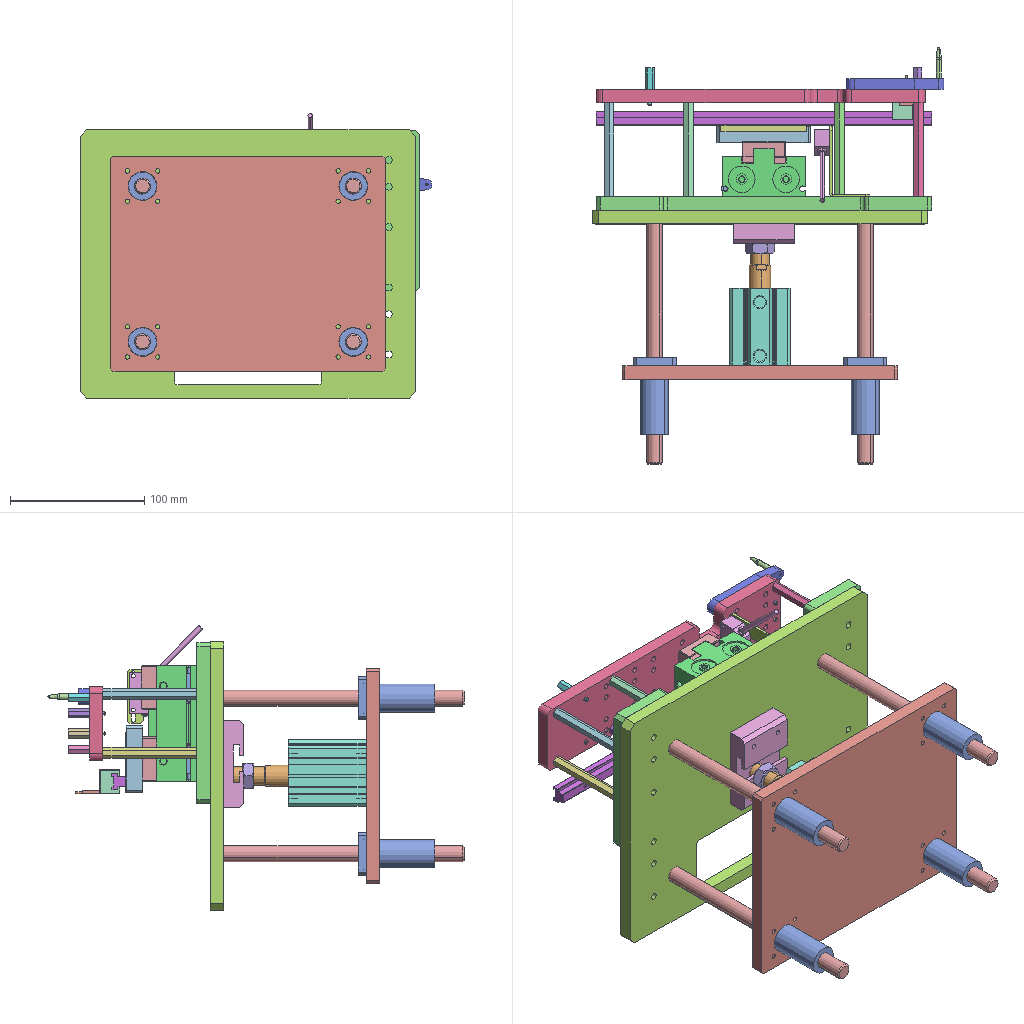Assembly | SolidWorks | 27 different items | 35 placed | box 262 x 310 x 212 mm
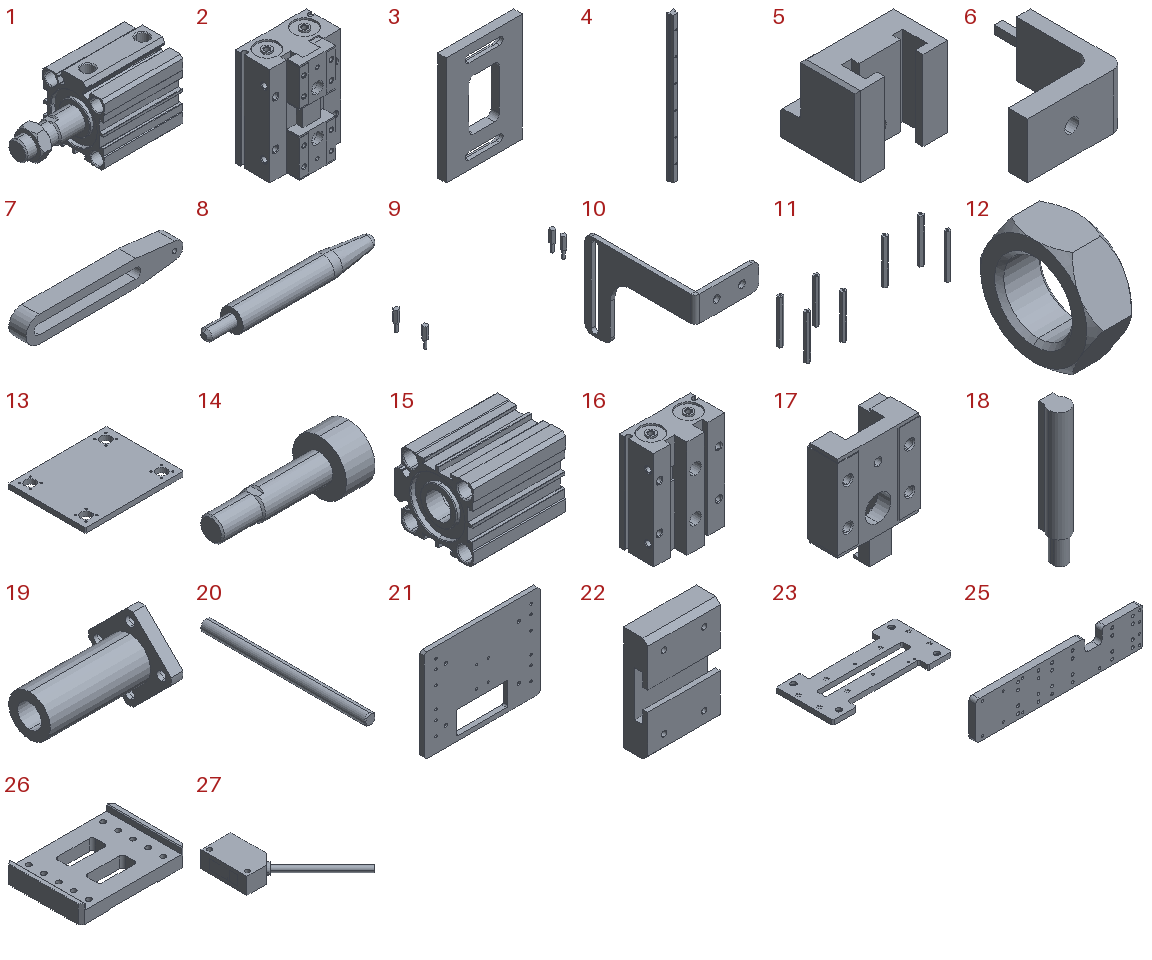Parts list (item | name | quantity | parent item | size | volume | features):
1 | (subassembly) | x1 | - | 99.4 x 45 x 49.5 mm | 88368 mm3 | -
2 | (subassembly) | x1 | - | 62.3 x 41 x 86.8 mm | 172165 mm3 | -
3 | - | x1 | - | 45 x 5 x 64 mm | 10150 mm3 | features ICE 2, Extrusion 1, Fillet 1
4 | - | x1 | - | 12 x 10 x 250 mm | 20615 mm3 | features Chamfer 1, Extrusion 1, HoleWzd 1, LPattern 1
5 | - | x1 | - | 18 x 15 x 15.5 mm | 2507 mm3 | features HoleWzd 2, Chamfer 1, Cut 1, Extrusion 1, Fillet 1
6 | - | x1 | - | 17.5 x 22 x 10 mm | 944.069 mm3 | features Extrusion 1, Fillet 1, HoleWzd 1, ICE 1
7 | - | x1 | - | 72.914 x 8 x 12 mm | 4560 mm3 | features Cut 2, Extrusion 1
8 | - | x1 | - | 30 x 4 x 4 mm | 285.134 mm3 | features Chamfer 1, ICE 1, Revolution 1
9 | - | x1 | - | 205.964 x 45 x 28 mm | 2330 mm3 | features Chamfer 4, Extrusion 1, ICE 1
10 | - | x1 | - | 30 x 52 x 40 mm | 2330 mm3 | features Fillet 2, ICE 2, FlatPattern 1, HoleWzd 1, SMBaseFlange 1, SheetMetal 1
11 | - | x1 | - | 237.4 x 52 x 72 mm | 21087 mm3 | features Extrusion 1, HoleWzd 1
12 | - | x1 | in 1 | 8 x 21.939 x 19 mm | 1486 mm3 | features BaseBody 1
13 | - | x1 | - | 205 x 160 x 10 mm | 312030 mm3 | features Chamfer 1, Cut 1, Extrusion 1, HoleWzd 1
14 | - | x1 | in 1 | 82 x 32 x 32 mm | 25673 mm3 | features BaseBody 1
15 | - | x1 | in 1 | 58 x 49.5 x 45 mm | 61209 mm3 | features BaseBody 1
16 | - | x1 | in 2 | 62 x 35.7 x 86 mm | 150902 mm3 | features BaseBody 1
17 | - | x2 | in 2 | 32 x 17.6 x 53.4 mm | 10272 mm3 | features BaseBody 1
18 | - | x2 | in 2 | 4 x 4.6 x 27 mm | 359.523 mm3 | features BaseBody 1
19 | - | x4 | - | 57 x 42 x 42 mm | 16451 mm3 | features HoleWzd 2, ICE 2, CirPattern 1, Extrusion 1
20 | - | x4 | - | 12 x 179 x 12 mm | 19967 mm3 | features Chamfer 1, Extrusion 1, HoleWzd 1
21 | - | x1 | - | 250 x 10 x 200 mm | 437930 mm3 | features HoleWzd 3, Cut 2, Chamfer 1, Extrusion 1, Fillet 1
22 | - | x1 | - | 45 x 15 x 65 mm | 35037 mm3 | features Chamfer 1, Extrusion 1, HoleWzd 1
23 | - | x1 | - | 250 x 120 x 10 mm | 200343 mm3 | features HoleWzd 3, Chamfer 1, Cut 1, Extrusion 1, Fillet 1
24 | - | x1 | - | - | - | -
25 | - | x1 | - | 245 x 10 x 55 mm | 124835 mm3 | features HoleWzd 2, Cut 1, Extrusion 1, LPattern 1
26 | - | x1 | - | 70 x 50 x 12 mm | 23909 mm3 | features Chamfer 2, ICE 2, Cut 1, Extrusion 1, Fillet 1, HoleWzd 1, LPattern 1, MirrorPattern 1
27 | - | x1 | - | 54.507 x 67.507 x 11.2 mm | 7170 mm3 | features BaseBody 3
Mates (type | each side: item.copy, entity, surface, feature):
In the top assembly
Concentric | 20.1 face cylinder Boss-Extrude1 | 19.1 face cylinder Boss-Extrude1
DistanceDim | 20.1 face plane Boss-Extrude1 | 13.1 face plane Boss-Extrude1
Concentric | 13.1 face cylinder Cut-Extrude1 | 19.1 face cylinder Boss-Extrude1
Parallel | 13.1 face plane Boss-Extrude1 | 19.1 face plane Cut-Extrude1
Coincident | 13.1 face plane Boss-Extrude1 | 19.1 face plane Boss-Extrude2
Width | 21.1 face plane Boss-Extrude1 | 21.1 face plane Boss-Extrude1 | 13.1 face plane Boss-Extrude1 | 13.1 face plane Boss-Extrude1 | 2 times
Coincident | 13.1 face plane Boss-Extrude1 | 15.1 face plane Input1
Width | 13.1 face plane Boss-Extrude1 | 13.1 face plane Boss-Extrude1 | 15.1 face plane Input1 | 15.1 face plane Input1 | 2 times
Coincident | 23.1 face plane Boss-Extrude1 | 25.1 face plane Boss-Extrude1
Width | 23.1 face plane Boss-Extrude1 | 23.1 face plane Boss-Extrude1 | 25.1 face plane Boss-Extrude1 | 25.1 face plane Boss-Extrude1
Coincident | 23.1 face plane Boss-Extrude1 | 16.1 face plane Input1
Width | 16.1 face plane Input1 | 16.1 face plane Input1 | 23.1 face plane Boss-Extrude1 | 23.1 face plane Boss-Extrude1
Width | 23.1 face plane Boss-Extrude1 | 23.1 face plane Boss-Extrude1 | 16.1 face plane Input1 | 16.1 face plane Input1
Coincident | 23.1 face plane Boss-Extrude1 | 10.1 face plane Base-Flange1 | 2 times
Coincident | 25.1 face plane Boss-Extrude1 | 7.1 face plane Boss-Extrude1
DistanceDim | 7.1 face plane Boss-Extrude1 | 25.1 face plane Boss-Extrude1
Coincident | 26.1 face plane Cut-Extrude1 | 3.1 face plane Boss-Extrude1 | 2 times
Parallel | 26.1 face plane Boss-Extrude1 | 3.1 face plane Boss-Extrude1
Coincident | 26.1 face plane Boss-Extrude1 | 3.1 face plane Boss-Extrude1
Width | 4.1 face plane Boss-Extrude1 | 4.1 face plane Boss-Extrude1 | 26.1 face plane Boss-Extrude1 | 26.1 face plane Boss-Extrude1
Width | 26.1 face plane Boss-Extrude1 | 26.1 face plane Boss-Extrude1 | 16.1 face plane Input1 | 16.1 face plane Input1
Coincident | 17.1 face plane Input1 | 26.1 face plane Cut-Extrude2
Width | 26.1 face plane Boss-Extrude1 | 26.1 face plane Boss-Extrude1 | 17.1 face plane Input1 | 17.1 face plane Input1
Coincident | 3.1 face plane Boss-Extrude1 | 4.1 face plane Boss-Extrude1
DistanceDim | 4.1 face plane Boss-Extrude1 | 3.1 face plane Boss-Extrude1
Coincident | 5.1 face plane Cut-Extrude1 | 6.1 face plane Boss-Extrude1 | 2 times
Coincident | 5.1 face plane Boss-Extrude1 | 6.1 face plane Boss-Extrude1
Concentric | 7.1 face cylinder Cut-Extrude1 | 8.1 face cylinder Revolve1
Coincident | 7.1 face plane Cut-Extrude1 | 8.1 face plane Revolve1
DistanceDim | 10.1 face plane Base-Flange1 | 16.1 face plane Input1
Coincident | 10.1 face plane Base-Flange1 | 27.1 face plane Input1
Parallel | 10.1 face plane Base-Flange1 | 27.1 face plane Input1
Slot | 27.1 face cylinder Input1 | 10.1 face cylinder Cut-Extrude1
Concentric | 13.1 face cylinder Cut-Extrude1 | 19.2 face cylinder Boss-Extrude1
Coincident | 13.1 face plane Boss-Extrude1 | 19.2 face plane Boss-Extrude2
Concentric | 19.2 face cylinder Boss-Extrude1 | 20.2 face cylinder Boss-Extrude1
Coincident | 21.1 face plane Boss-Extrude1 | 20.2 face plane Boss-Extrude1
Concentric | 13.1 face cylinder Cut-Extrude1 | 19.3 face cylinder Boss-Extrude1
Coincident | 13.1 face plane Boss-Extrude1 | 19.3 face plane Boss-Extrude2
Parallel | 13.1 face plane Boss-Extrude1 | 19.3 face plane Cut-Extrude1
Concentric | 13.1 face cylinder Cut-Extrude1 | 19.4 face cylinder Boss-Extrude1
Coincident | 13.1 face plane Boss-Extrude1 | 19.4 face plane Boss-Extrude2
Concentric | 19.3 face cylinder Boss-Extrude1 | 20.3 face cylinder Boss-Extrude1
Coincident | 21.1 face plane Boss-Extrude1 | 20.3 face plane Boss-Extrude1
Concentric | 19.4 face cylinder Boss-Extrude1 | 20.4 face cylinder Boss-Extrude1
Coincident | 21.1 face plane Boss-Extrude1 | 20.4 face plane Boss-Extrude1
In subassembly 1
Concentric | 14.1 face cylinder Input1 | 12.1 face cylinder Input1
Concentric | 15.2 face cylinder Input1 | 14.1 face cylinder Input1
Width | 15.2 face plane Input1 | 15.2 face plane Input1 | 14.1 face plane Input1 | 14.1 face plane Input1